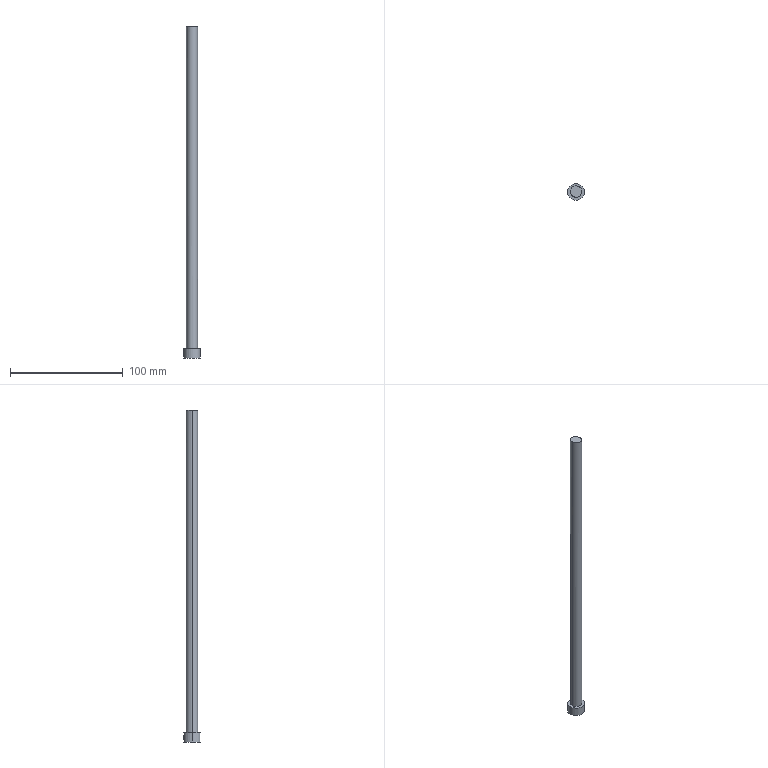Part | Creo | 1 solid | 10 faces | box 15 x 15 x 294.447 mm | volume 23843 mm3 | cylinder 6 | plane 4 | commonest cylinder face diameters 3 x2 10 x2 15 x2
STEP:
#1=CARTESIAN_POINT('',(30.,201.,-252.5));
#2=VERTEX_POINT('',#1);
#3=CARTESIAN_POINT('',(40.,201.,-252.5));
#4=VERTEX_POINT('',#3);
#5=CARTESIAN_POINT('',(35.,201.,-252.5));
#6=DIRECTION('',(0.,0.,-1.));
#7=DIRECTION('',(-1.,0.,0.));
#8=AXIS2_PLACEMENT_3D('',#5,#6,#7);
#9=CIRCLE('',#8,5.);
#10=EDGE_CURVE('',#2,#4,#9,.T.);
#11=ORIENTED_EDGE('',*,*,#10,.T.);
#12=CARTESIAN_POINT('',(40.,201.,33.565));
#13=VERTEX_POINT('',#12);
#14=CARTESIAN_POINT('',(40.,201.,33.565));
#15=DIRECTION('',(0.,0.,-1.));
#16=VECTOR('',#15,286.065);
#17=LINE('',#14,#16);
#18=EDGE_CURVE('',#13,#4,#17,.T.);
#19=ORIENTED_EDGE('',*,*,#18,.F.);
#20=CARTESIAN_POINT('',(30.,201.,33.947));
#21=VERTEX_POINT('',#20);
#22=CARTESIAN_POINT('',(40.,201.,33.565));
#23=CARTESIAN_POINT('',(40.,201.589,33.565));
#24=CARTESIAN_POINT('',(39.785,202.862,33.573));
#25=CARTESIAN_POINT('',(38.645,204.641,33.617));
#26=CARTESIAN_POINT('',(36.85,205.786,33.685));
#27=CARTESIAN_POINT('',(35.,206.107,33.756));
#28=CARTESIAN_POINT('',(33.15,205.786,33.827));
#29=CARTESIAN_POINT('',(31.355,204.641,33.895));
#30=CARTESIAN_POINT('',(30.215,202.862,33.939));
#31=CARTESIAN_POINT('',(30.,201.589,33.947));
#32=CARTESIAN_POINT('',(30.,201.,33.947));
#33=B_SPLINE_CURVE_WITH_KNOTS('',3,(#22,#23,#24,#25,#26,#27,#28,#29,#30,#31,#32),.UNSPECIFIED.,.F.,.F.,(4,1,1,1,1,1,1,1,4),(0.,0.125,0.25,0.375,0.5,0.625,0.75,0.875,1.),.UNSPECIFIED.);
#34=EDGE_CURVE('',#13,#21,#33,.T.);
#35=ORIENTED_EDGE('',*,*,#34,.T.);
#36=CARTESIAN_POINT('',(30.,201.,33.947));
#37=DIRECTION('',(0.,0.,-1.));
#38=VECTOR('',#37,286.447);
#39=LINE('',#36,#38);
#40=EDGE_CURVE('',#21,#2,#39,.T.);
#41=ORIENTED_EDGE('',*,*,#40,.T.);
#42=EDGE_LOOP('',(#11,#19,#35,#41));
#43=FACE_OUTER_BOUND('',#42,.F.);
#44=CARTESIAN_POINT('',(35.,201.,135.));
#45=DIRECTION('',(0.,0.,-1.));
#46=DIRECTION('',(-1.,0.,0.));
#47=AXIS2_PLACEMENT_3D('',#44,#45,#46);
#48=CYLINDRICAL_SURFACE('',#47,5.);
#49=ADVANCED_FACE('',(#43),#48,.T.);
#50=CARTESIAN_POINT('',(27.5,201.,-252.5));
#51=VERTEX_POINT('',#50);
#52=CARTESIAN_POINT('',(42.5,201.,-252.5));
#53=VERTEX_POINT('',#52);
#54=CARTESIAN_POINT('',(35.,201.,-252.5));
#55=DIRECTION('',(0.,0.,1.));
#56=DIRECTION('',(-1.,0.,0.));
#57=AXIS2_PLACEMENT_3D('',#54,#55,#56);
#58=CIRCLE('',#57,7.5);
#59=EDGE_CURVE('',#51,#53,#58,.T.);
#60=ORIENTED_EDGE('',*,*,#59,.F.);
#61=CARTESIAN_POINT('',(35.,201.,-252.5));
#62=DIRECTION('',(0.,0.,1.));
#63=DIRECTION('',(1.,0.,0.));
#64=AXIS2_PLACEMENT_3D('',#61,#62,#63);
#65=CIRCLE('',#64,7.5);
#66=EDGE_CURVE('',#53,#51,#65,.T.);
#67=ORIENTED_EDGE('',*,*,#66,.F.);
#68=EDGE_LOOP('',(#60,#67));
#69=FACE_OUTER_BOUND('',#68,.F.);
#70=ORIENTED_EDGE('',*,*,#10,.F.);
#71=CARTESIAN_POINT('',(35.,201.,-252.5));
#72=DIRECTION('',(0.,0.,-1.));
#73=DIRECTION('',(1.,0.,0.));
#74=AXIS2_PLACEMENT_3D('',#71,#72,#73);
#75=CIRCLE('',#74,5.);
#76=EDGE_CURVE('',#4,#2,#75,.T.);
#77=ORIENTED_EDGE('',*,*,#76,.F.);
#78=EDGE_LOOP('',(#70,#77));
#79=FACE_BOUND('',#78,.F.);
#80=CARTESIAN_POINT('',(35.,201.,-252.5));
#81=DIRECTION('',(0.,0.,1.));
#82=DIRECTION('',(-1.,0.,0.));
#83=AXIS2_PLACEMENT_3D('',#80,#81,#82);
#84=PLANE('',#83);
#85=ADVANCED_FACE('',(#69,#79),#84,.T.);
#86=ORIENTED_EDGE('',*,*,#76,.T.);
#87=ORIENTED_EDGE('',*,*,#40,.F.);
#88=CARTESIAN_POINT('',(30.,201.,33.947));
#89=CARTESIAN_POINT('',(30.,200.411,33.947));
#90=CARTESIAN_POINT('',(30.215,199.138,33.939));
#91=CARTESIAN_POINT('',(31.355,197.359,33.895));
#92=CARTESIAN_POINT('',(33.15,196.214,33.827));
#93=CARTESIAN_POINT('',(35.,195.893,33.756));
#94=CARTESIAN_POINT('',(36.85,196.214,33.685));
#95=CARTESIAN_POINT('',(38.645,197.359,33.617));
#96=CARTESIAN_POINT('',(39.785,199.138,33.573));
#97=CARTESIAN_POINT('',(40.,200.411,33.565));
#98=CARTESIAN_POINT('',(40.,201.,33.565));
#99=B_SPLINE_CURVE_WITH_KNOTS('',3,(#88,#89,#90,#91,#92,#93,#94,#95,#96,#97,#98),.UNSPECIFIED.,.F.,.F.,(4,1,1,1,1,1,1,1,4),(0.,0.125,0.25,0.375,0.5,0.625,0.75,0.875,1.),.UNSPECIFIED.);
#100=EDGE_CURVE('',#21,#13,#99,.T.);
#101=ORIENTED_EDGE('',*,*,#100,.T.);
#102=ORIENTED_EDGE('',*,*,#18,.T.);
#103=EDGE_LOOP('',(#86,#87,#101,#102));
#104=FACE_OUTER_BOUND('',#103,.F.);
#105=CARTESIAN_POINT('',(35.,201.,135.));
#106=DIRECTION('',(0.,0.,-1.));
#107=DIRECTION('',(-1.,0.,0.));
#108=AXIS2_PLACEMENT_3D('',#105,#106,#107);
#109=CYLINDRICAL_SURFACE('',#108,5.);
#110=ADVANCED_FACE('',(#104),#109,.T.);
#111=ORIENTED_EDGE('',*,*,#34,.F.);
#112=ORIENTED_EDGE('',*,*,#100,.F.);
#113=EDGE_LOOP('',(#111,#112));
#114=FACE_OUTER_BOUND('',#113,.F.);
#115=CARTESIAN_POINT('',(0.9569,33.474,35.055));
#116=DIRECTION('',(0.03814,0.,0.9993));
#117=DIRECTION('',(0.9993,0.,-0.03814));
#118=AXIS2_PLACEMENT_3D('',#115,#116,#117);
#119=PLANE('',#118);
#120=ADVANCED_FACE('',(#114),#119,.T.);
#121=ORIENTED_EDGE('',*,*,#59,.T.);
#122=CARTESIAN_POINT('',(42.5,201.,-260.5));
#123=VERTEX_POINT('',#122);
#124=CARTESIAN_POINT('',(42.5,201.,-260.5));
#125=DIRECTION('',(0.,0.,1.));
#126=VECTOR('',#125,8.);
#127=LINE('',#124,#126);
#128=EDGE_CURVE('',#123,#53,#127,.T.);
#129=ORIENTED_EDGE('',*,*,#128,.F.);
#130=CARTESIAN_POINT('',(27.5,201.,-260.5));
#131=VERTEX_POINT('',#130);
#132=CARTESIAN_POINT('',(35.,201.,-260.5));
#133=DIRECTION('',(0.,0.,-1.));
#134=DIRECTION('',(1.,0.,0.));
#135=AXIS2_PLACEMENT_3D('',#132,#133,#134);
#136=CIRCLE('',#135,7.5);
#137=EDGE_CURVE('',#123,#131,#136,.T.);
#138=ORIENTED_EDGE('',*,*,#137,.T.);
#139=CARTESIAN_POINT('',(27.5,201.,-260.5));
#140=DIRECTION('',(0.,0.,1.));
#141=VECTOR('',#140,8.);
#142=LINE('',#139,#141);
#143=EDGE_CURVE('',#131,#51,#142,.T.);
#144=ORIENTED_EDGE('',*,*,#143,.T.);
#145=EDGE_LOOP('',(#121,#129,#138,#144));
#146=FACE_OUTER_BOUND('',#145,.F.);
#147=CARTESIAN_POINT('',(35.,201.,-260.5));
#148=DIRECTION('',(0.,0.,1.));
#149=DIRECTION('',(-1.,0.,0.));
#150=AXIS2_PLACEMENT_3D('',#147,#148,#149);
#151=CYLINDRICAL_SURFACE('',#150,7.5);
#152=ADVANCED_FACE('',(#146),#151,.T.);
#153=ORIENTED_EDGE('',*,*,#66,.T.);
#154=ORIENTED_EDGE('',*,*,#143,.F.);
#155=CARTESIAN_POINT('',(35.,201.,-260.5));
#156=DIRECTION('',(0.,0.,-1.));
#157=DIRECTION('',(-1.,0.,0.));
#158=AXIS2_PLACEMENT_3D('',#155,#156,#157);
#159=CIRCLE('',#158,7.5);
#160=EDGE_CURVE('',#131,#123,#159,.T.);
#161=ORIENTED_EDGE('',*,*,#160,.T.);
#162=ORIENTED_EDGE('',*,*,#128,.T.);
#163=EDGE_LOOP('',(#153,#154,#161,#162));
#164=FACE_OUTER_BOUND('',#163,.F.);
#165=CARTESIAN_POINT('',(35.,208.5,-258.));
#166=VERTEX_POINT('',#165);
#167=CARTESIAN_POINT('',(35.,208.5,-255.));
#168=VERTEX_POINT('',#167);
#169=CARTESIAN_POINT('',(35.,208.5,-258.));
#170=CARTESIAN_POINT('',(35.205,208.5,-258.));
#171=CARTESIAN_POINT('',(35.583,208.484,-257.922));
#172=CARTESIAN_POINT('',(36.09,208.425,-257.589));
#173=CARTESIAN_POINT('',(36.424,208.365,-257.085));
#174=CARTESIAN_POINT('',(36.539,208.34,-256.497));
#175=CARTESIAN_POINT('',(36.422,208.365,-255.912));
#176=CARTESIAN_POINT('',(36.091,208.425,-255.413));
#177=CARTESIAN_POINT('',(35.585,208.484,-255.078));
#178=CARTESIAN_POINT('',(35.206,208.5,-255.));
#179=CARTESIAN_POINT('',(35.,208.5,-255.));
#180=B_SPLINE_CURVE_WITH_KNOTS('',3,(#169,#170,#171,#172,#173,#174,#175,#176,#177,#178,#179),.UNSPECIFIED.,.F.,.F.,(4,1,1,1,1,1,1,1,4),(0.,0.125,0.25,0.375,0.5,0.625,0.75,0.875,1.),.UNSPECIFIED.);
#181=EDGE_CURVE('',#166,#168,#180,.T.);
#182=ORIENTED_EDGE('',*,*,#181,.F.);
#183=CARTESIAN_POINT('',(35.,208.5,-255.));
#184=CARTESIAN_POINT('',(34.794,208.5,-255.));
#185=CARTESIAN_POINT('',(34.415,208.484,-255.078));
#186=CARTESIAN_POINT('',(33.907,208.424,-255.414));
#187=CARTESIAN_POINT('',(33.576,208.364,-255.917));
#188=CARTESIAN_POINT('',(33.461,208.34,-256.506));
#189=CARTESIAN_POINT('',(33.579,208.365,-257.089));
#190=CARTESIAN_POINT('',(33.908,208.424,-257.586));
#191=CARTESIAN_POINT('',(34.414,208.484,-257.922));
#192=CARTESIAN_POINT('',(34.794,208.5,-258.));
#193=CARTESIAN_POINT('',(35.,208.5,-258.));
#194=B_SPLINE_CURVE_WITH_KNOTS('',3,(#183,#184,#185,#186,#187,#188,#189,#190,#191,#192,#193),.UNSPECIFIED.,.F.,.F.,(4,1,1,1,1,1,1,1,4),(0.,0.125,0.25,0.375,0.5,0.625,0.75,0.875,1.),.UNSPECIFIED.);
#195=EDGE_CURVE('',#168,#166,#194,.T.);
#196=ORIENTED_EDGE('',*,*,#195,.F.);
#197=EDGE_LOOP('',(#182,#196));
#198=FACE_BOUND('',#197,.F.);
#199=CARTESIAN_POINT('',(35.,201.,-260.5));
#200=DIRECTION('',(0.,0.,1.));
#201=DIRECTION('',(-1.,0.,0.));
#202=AXIS2_PLACEMENT_3D('',#199,#200,#201);
#203=CYLINDRICAL_SURFACE('',#202,7.5);
#204=ADVANCED_FACE('',(#164,#198),#203,.T.);
#205=ORIENTED_EDGE('',*,*,#181,.T.);
#206=CARTESIAN_POINT('',(35.,201.,-255.));
#207=VERTEX_POINT('',#206);
#208=CARTESIAN_POINT('',(35.,201.,-255.));
#209=DIRECTION('',(-0.000000004,1.,-0.000006083));
#210=VECTOR('',#209,7.5);
#211=LINE('',#208,#210);
#212=EDGE_CURVE('',#207,#168,#211,.T.);
#213=ORIENTED_EDGE('',*,*,#212,.F.);
#214=CARTESIAN_POINT('',(35.,201.,-258.));
#215=VERTEX_POINT('',#214);
#216=CARTESIAN_POINT('',(35.,201.,-256.5));
#217=DIRECTION('',(0.,1.,0.));
#218=DIRECTION('',(0.,0.,1.));
#219=AXIS2_PLACEMENT_3D('',#216,#217,#218);
#220=CIRCLE('',#219,1.5);
#221=EDGE_CURVE('',#207,#215,#220,.T.);
#222=ORIENTED_EDGE('',*,*,#221,.T.);
#223=CARTESIAN_POINT('',(35.,201.,-258.));
#224=DIRECTION('',(0.,1.,0.));
#225=VECTOR('',#224,7.5);
#226=LINE('',#223,#225);
#227=EDGE_CURVE('',#215,#166,#226,.T.);
#228=ORIENTED_EDGE('',*,*,#227,.T.);
#229=EDGE_LOOP('',(#205,#213,#222,#228));
#230=FACE_OUTER_BOUND('',#229,.F.);
#231=CARTESIAN_POINT('',(35.,201.,-256.5));
#232=DIRECTION('',(0.,1.,0.));
#233=DIRECTION('',(0.,0.,-1.));
#234=AXIS2_PLACEMENT_3D('',#231,#232,#233);
#235=CYLINDRICAL_SURFACE('',#234,1.5);
#236=ADVANCED_FACE('',(#230),#235,.F.);
#237=ORIENTED_EDGE('',*,*,#195,.T.);
#238=ORIENTED_EDGE('',*,*,#227,.F.);
#239=CARTESIAN_POINT('',(35.,201.,-256.5));
#240=DIRECTION('',(0.,1.,0.));
#241=DIRECTION('',(0.,0.,-1.));
#242=AXIS2_PLACEMENT_3D('',#239,#240,#241);
#243=CIRCLE('',#242,1.5);
#244=EDGE_CURVE('',#215,#207,#243,.T.);
#245=ORIENTED_EDGE('',*,*,#244,.T.);
#246=ORIENTED_EDGE('',*,*,#212,.T.);
#247=EDGE_LOOP('',(#237,#238,#245,#246));
#248=FACE_OUTER_BOUND('',#247,.F.);
#249=CARTESIAN_POINT('',(35.,201.,-256.5));
#250=DIRECTION('',(0.,1.,0.));
#251=DIRECTION('',(0.,0.,-1.));
#252=AXIS2_PLACEMENT_3D('',#249,#250,#251);
#253=CYLINDRICAL_SURFACE('',#252,1.5);
#254=ADVANCED_FACE('',(#248),#253,.F.);
#255=ORIENTED_EDGE('',*,*,#244,.F.);
#256=ORIENTED_EDGE('',*,*,#221,.F.);
#257=EDGE_LOOP('',(#255,#256));
#258=FACE_OUTER_BOUND('',#257,.F.);
#259=CARTESIAN_POINT('',(35.,201.,-256.5));
#260=DIRECTION('',(0.,-1.,0.));
#261=DIRECTION('',(0.,0.,1.));
#262=AXIS2_PLACEMENT_3D('',#259,#260,#261);
#263=PLANE('',#262);
#264=ADVANCED_FACE('',(#258),#263,.F.);
#265=ORIENTED_EDGE('',*,*,#137,.F.);
#266=ORIENTED_EDGE('',*,*,#160,.F.);
#267=EDGE_LOOP('',(#265,#266));
#268=FACE_OUTER_BOUND('',#267,.F.);
#269=CARTESIAN_POINT('',(72.286,343.015,-260.5));
#270=DIRECTION('',(0.,0.,-1.));
#271=DIRECTION('',(1.,0.,0.));
#272=AXIS2_PLACEMENT_3D('',#269,#270,#271);
#273=PLANE('',#272);
#274=ADVANCED_FACE('',(#268),#273,.T.);
#275=CLOSED_SHELL('',(#49,#85,#110,#120,#152,#204,#236,#254,#264,#274));
#276=MANIFOLD_SOLID_BREP('',#275);
#277=(LENGTH_UNIT()NAMED_UNIT(*)SI_UNIT(.MILLI.,.METRE.));
#278=UNCERTAINTY_MEASURE_WITH_UNIT(LENGTH_MEASURE(0.02952),#277,'','');
#279=(NAMED_UNIT(*)PLANE_ANGLE_UNIT()SI_UNIT($,.RADIAN.));
#280=PLANE_ANGLE_MEASURE_WITH_UNIT(PLANE_ANGLE_MEASURE(0.01745),#279);
#281=(CONVERSION_BASED_UNIT('DEGREE',#280)NAMED_UNIT(*)PLANE_ANGLE_UNIT());
#282=(NAMED_UNIT(*)SI_UNIT($,.STERADIAN.)SOLID_ANGLE_UNIT());
#283=(GEOMETRIC_REPRESENTATION_CONTEXT(3)GLOBAL_UNCERTAINTY_ASSIGNED_CONTEXT((#278))GLOBAL_UNIT_ASSIGNED_CONTEXT((#277,#281,#282))REPRESENTATION_CONTEXT('',''));
#284=ADVANCED_BREP_SHAPE_REPRESENTATION('',(#276),#283);